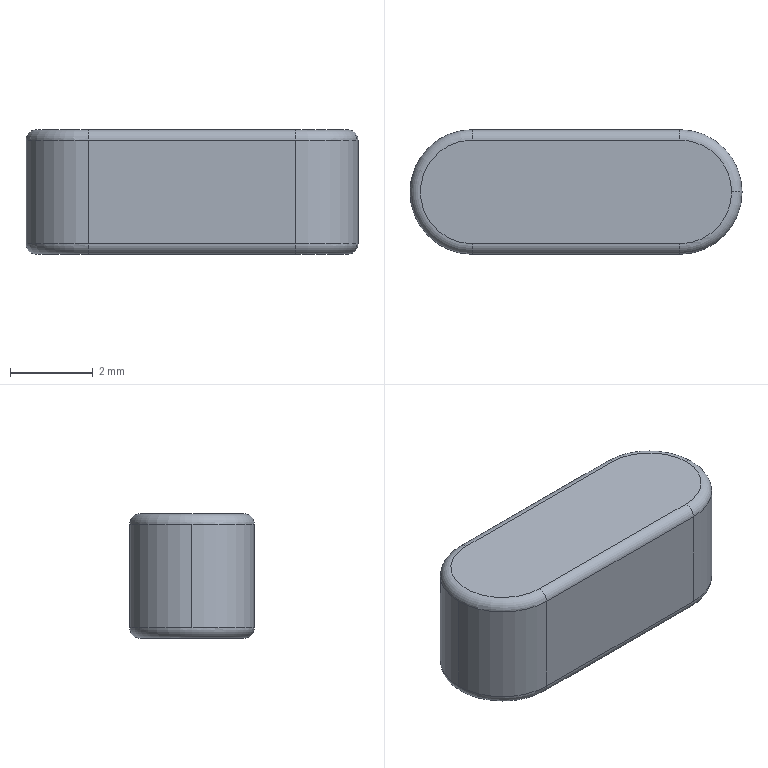Part | SolidWorks | features Extrusion 1, Fillet 1 | 1 solid | 17 faces | box 8 x 3 x 3 mm | volume 65.694 mm3 | cylinder 7 | torus 6 | plane 4 | commonest cylinder face diameters 0.5 x4 3 x3
STEP:
#1=CARTESIAN_POINT('',(3.75,0.,0.));
#2=VERTEX_POINT('',#1);
#3=CARTESIAN_POINT('',(2.5,-1.25,0.));
#4=VERTEX_POINT('',#3);
#5=CARTESIAN_POINT('',(2.5,0.,0.));
#6=DIRECTION('',(0.,0.,-1.));
#7=DIRECTION('',(1.,0.,0.));
#8=AXIS2_PLACEMENT_3D('',#5,#6,#7);
#9=CIRCLE('',#8,1.25);
#10=EDGE_CURVE('',#2,#4,#9,.T.);
#11=ORIENTED_EDGE('',*,*,#10,.F.);
#12=CARTESIAN_POINT('',(4.,0.,0.25));
#13=VERTEX_POINT('',#12);
#14=CARTESIAN_POINT('',(3.75,0.,0.25));
#15=DIRECTION('',(0.,-1.,0.));
#16=DIRECTION('',(0.,0.,-1.));
#17=AXIS2_PLACEMENT_3D('',#14,#15,#16);
#18=CIRCLE('',#17,0.25);
#19=EDGE_CURVE('',#2,#13,#18,.T.);
#20=ORIENTED_EDGE('',*,*,#19,.T.);
#21=CARTESIAN_POINT('',(2.5,-1.5,0.25));
#22=VERTEX_POINT('',#21);
#23=CARTESIAN_POINT('',(2.5,0.,0.25));
#24=DIRECTION('',(0.,0.,1.));
#25=DIRECTION('',(1.,0.,0.));
#26=AXIS2_PLACEMENT_3D('',#23,#24,#25);
#27=CIRCLE('',#26,1.5);
#28=EDGE_CURVE('',#22,#13,#27,.T.);
#29=ORIENTED_EDGE('',*,*,#28,.F.);
#30=CARTESIAN_POINT('',(2.5,-1.25,0.25));
#31=DIRECTION('',(1.,0.,0.));
#32=DIRECTION('',(0.,0.,-1.));
#33=AXIS2_PLACEMENT_3D('',#30,#31,#32);
#34=CIRCLE('',#33,0.25);
#35=EDGE_CURVE('',#22,#4,#34,.T.);
#36=ORIENTED_EDGE('',*,*,#35,.T.);
#37=EDGE_LOOP('',(#11,#20,#29,#36));
#38=FACE_OUTER_BOUND('',#37,.T.);
#39=CARTESIAN_POINT('',(2.5,0.,0.25));
#40=DIRECTION('',(0.,0.,1.));
#41=DIRECTION('',(1.,0.,0.));
#42=AXIS2_PLACEMENT_3D('',#39,#40,#41);
#43=TOROIDAL_SURFACE('',#42,1.25,0.25);
#44=ADVANCED_FACE('',(#38),#43,.T.);
#45=CARTESIAN_POINT('',(4.,0.,2.75));
#46=VERTEX_POINT('',#45);
#47=CARTESIAN_POINT('',(2.5,-1.5,2.75));
#48=VERTEX_POINT('',#47);
#49=CARTESIAN_POINT('',(2.5,0.,2.75));
#50=DIRECTION('',(0.,0.,-1.));
#51=DIRECTION('',(1.,0.,0.));
#52=AXIS2_PLACEMENT_3D('',#49,#50,#51);
#53=CIRCLE('',#52,1.5);
#54=EDGE_CURVE('',#46,#48,#53,.T.);
#55=ORIENTED_EDGE('',*,*,#54,.F.);
#56=CARTESIAN_POINT('',(3.75,0.,3.));
#57=VERTEX_POINT('',#56);
#58=CARTESIAN_POINT('',(3.75,0.,2.75));
#59=DIRECTION('',(0.,-1.,0.));
#60=DIRECTION('',(0.,0.,-1.));
#61=AXIS2_PLACEMENT_3D('',#58,#59,#60);
#62=CIRCLE('',#61,0.25);
#63=EDGE_CURVE('',#46,#57,#62,.T.);
#64=ORIENTED_EDGE('',*,*,#63,.T.);
#65=CARTESIAN_POINT('',(2.5,-1.25,3.));
#66=VERTEX_POINT('',#65);
#67=CARTESIAN_POINT('',(2.5,0.,3.));
#68=DIRECTION('',(0.,0.,1.));
#69=DIRECTION('',(1.,0.,0.));
#70=AXIS2_PLACEMENT_3D('',#67,#68,#69);
#71=CIRCLE('',#70,1.25);
#72=EDGE_CURVE('',#66,#57,#71,.T.);
#73=ORIENTED_EDGE('',*,*,#72,.F.);
#74=CARTESIAN_POINT('',(2.5,-1.25,2.75));
#75=DIRECTION('',(1.,0.,0.));
#76=DIRECTION('',(0.,0.,-1.));
#77=AXIS2_PLACEMENT_3D('',#74,#75,#76);
#78=CIRCLE('',#77,0.25);
#79=EDGE_CURVE('',#66,#48,#78,.T.);
#80=ORIENTED_EDGE('',*,*,#79,.T.);
#81=EDGE_LOOP('',(#55,#64,#73,#80));
#82=FACE_OUTER_BOUND('',#81,.T.);
#83=CARTESIAN_POINT('',(2.5,0.,2.75));
#84=DIRECTION('',(0.,0.,1.));
#85=DIRECTION('',(1.,0.,0.));
#86=AXIS2_PLACEMENT_3D('',#83,#84,#85);
#87=TOROIDAL_SURFACE('',#86,1.25,0.25);
#88=ADVANCED_FACE('',(#82),#87,.T.);
#89=CARTESIAN_POINT('',(-2.5,-1.5,2.75));
#90=VERTEX_POINT('',#89);
#91=CARTESIAN_POINT('',(-4.,0.,2.75));
#92=VERTEX_POINT('',#91);
#93=CARTESIAN_POINT('',(-2.5,0.,2.75));
#94=DIRECTION('',(0.,0.,-1.));
#95=DIRECTION('',(1.,0.,0.));
#96=AXIS2_PLACEMENT_3D('',#93,#94,#95);
#97=CIRCLE('',#96,1.5);
#98=EDGE_CURVE('',#90,#92,#97,.T.);
#99=ORIENTED_EDGE('',*,*,#98,.T.);
#100=CARTESIAN_POINT('',(-4.,0.,0.25));
#101=VERTEX_POINT('',#100);
#102=CARTESIAN_POINT('',(-4.,0.,3.));
#103=DIRECTION('',(0.,0.,-1.));
#104=VECTOR('',#103,1000.);
#105=LINE('',#102,#104);
#106=EDGE_CURVE('',#92,#101,#105,.T.);
#107=ORIENTED_EDGE('',*,*,#106,.T.);
#108=CARTESIAN_POINT('',(-2.5,-1.5,0.25));
#109=VERTEX_POINT('',#108);
#110=CARTESIAN_POINT('',(-2.5,0.,0.25));
#111=DIRECTION('',(0.,0.,1.));
#112=DIRECTION('',(1.,0.,0.));
#113=AXIS2_PLACEMENT_3D('',#110,#111,#112);
#114=CIRCLE('',#113,1.5);
#115=EDGE_CURVE('',#101,#109,#114,.T.);
#116=ORIENTED_EDGE('',*,*,#115,.T.);
#117=CARTESIAN_POINT('',(-2.5,-1.5,3.));
#118=DIRECTION('',(0.,0.,-1.));
#119=VECTOR('',#118,1000.);
#120=LINE('',#117,#119);
#121=EDGE_CURVE('',#90,#109,#120,.T.);
#122=ORIENTED_EDGE('',*,*,#121,.F.);
#123=EDGE_LOOP('',(#99,#107,#116,#122));
#124=FACE_OUTER_BOUND('',#123,.T.);
#125=CARTESIAN_POINT('',(-2.5,0.,3.));
#126=DIRECTION('',(0.,0.,-1.));
#127=DIRECTION('',(-1.,0.,0.));
#128=AXIS2_PLACEMENT_3D('',#125,#126,#127);
#129=CYLINDRICAL_SURFACE('',#128,1.5);
#130=ADVANCED_FACE('',(#124),#129,.T.);
#131=ORIENTED_EDGE('',*,*,#106,.F.);
#132=CARTESIAN_POINT('',(-2.5,1.5,2.75));
#133=VERTEX_POINT('',#132);
#134=CARTESIAN_POINT('',(-2.5,0.,2.75));
#135=DIRECTION('',(0.,0.,-1.));
#136=DIRECTION('',(1.,0.,0.));
#137=AXIS2_PLACEMENT_3D('',#134,#135,#136);
#138=CIRCLE('',#137,1.5);
#139=EDGE_CURVE('',#92,#133,#138,.T.);
#140=ORIENTED_EDGE('',*,*,#139,.T.);
#141=CARTESIAN_POINT('',(-2.5,1.5,0.25));
#142=VERTEX_POINT('',#141);
#143=CARTESIAN_POINT('',(-2.5,1.5,3.));
#144=DIRECTION('',(0.,0.,-1.));
#145=VECTOR('',#144,1000.);
#146=LINE('',#143,#145);
#147=EDGE_CURVE('',#133,#142,#146,.T.);
#148=ORIENTED_EDGE('',*,*,#147,.T.);
#149=CARTESIAN_POINT('',(-2.5,0.,0.25));
#150=DIRECTION('',(0.,0.,1.));
#151=DIRECTION('',(1.,0.,0.));
#152=AXIS2_PLACEMENT_3D('',#149,#150,#151);
#153=CIRCLE('',#152,1.5);
#154=EDGE_CURVE('',#142,#101,#153,.T.);
#155=ORIENTED_EDGE('',*,*,#154,.T.);
#156=EDGE_LOOP('',(#131,#140,#148,#155));
#157=FACE_OUTER_BOUND('',#156,.T.);
#158=CARTESIAN_POINT('',(-2.5,0.,3.));
#159=DIRECTION('',(0.,0.,-1.));
#160=DIRECTION('',(-1.,0.,0.));
#161=AXIS2_PLACEMENT_3D('',#158,#159,#160);
#162=CYLINDRICAL_SURFACE('',#161,1.5);
#163=ADVANCED_FACE('',(#157),#162,.T.);
#164=CARTESIAN_POINT('',(2.5,-1.5,3.));
#165=DIRECTION('',(0.,0.,-1.));
#166=VECTOR('',#165,1000.);
#167=LINE('',#164,#166);
#168=EDGE_CURVE('',#48,#22,#167,.T.);
#169=ORIENTED_EDGE('',*,*,#168,.F.);
#170=CARTESIAN_POINT('',(-2.5,-1.5,2.75));
#171=DIRECTION('',(-1.,0.,0.));
#172=VECTOR('',#171,1000.);
#173=LINE('',#170,#172);
#174=EDGE_CURVE('',#48,#90,#173,.T.);
#175=ORIENTED_EDGE('',*,*,#174,.T.);
#176=ORIENTED_EDGE('',*,*,#121,.T.);
#177=CARTESIAN_POINT('',(-2.5,-1.5,0.25));
#178=DIRECTION('',(1.,0.,0.));
#179=VECTOR('',#178,1000.);
#180=LINE('',#177,#179);
#181=EDGE_CURVE('',#109,#22,#180,.T.);
#182=ORIENTED_EDGE('',*,*,#181,.T.);
#183=EDGE_LOOP('',(#169,#175,#176,#182));
#184=FACE_OUTER_BOUND('',#183,.T.);
#185=CARTESIAN_POINT('',(-2.5,-1.5,3.));
#186=DIRECTION('',(0.,1.,0.));
#187=DIRECTION('',(-1.,0.,0.));
#188=AXIS2_PLACEMENT_3D('',#185,#186,#187);
#189=PLANE('',#188);
#190=ADVANCED_FACE('',(#184),#189,.F.);
#191=CARTESIAN_POINT('',(2.5,1.5,2.75));
#192=VERTEX_POINT('',#191);
#193=CARTESIAN_POINT('',(2.5,1.5,0.25));
#194=VERTEX_POINT('',#193);
#195=CARTESIAN_POINT('',(2.5,1.5,3.));
#196=DIRECTION('',(0.,0.,-1.));
#197=VECTOR('',#196,1000.);
#198=LINE('',#195,#197);
#199=EDGE_CURVE('',#192,#194,#198,.T.);
#200=ORIENTED_EDGE('',*,*,#199,.F.);
#201=CARTESIAN_POINT('',(2.5,0.,2.75));
#202=DIRECTION('',(0.,0.,-1.));
#203=DIRECTION('',(1.,0.,0.));
#204=AXIS2_PLACEMENT_3D('',#201,#202,#203);
#205=CIRCLE('',#204,1.5);
#206=EDGE_CURVE('',#192,#46,#205,.T.);
#207=ORIENTED_EDGE('',*,*,#206,.T.);
#208=ORIENTED_EDGE('',*,*,#54,.T.);
#209=ORIENTED_EDGE('',*,*,#168,.T.);
#210=ORIENTED_EDGE('',*,*,#28,.T.);
#211=CARTESIAN_POINT('',(2.5,0.,0.25));
#212=DIRECTION('',(0.,0.,1.));
#213=DIRECTION('',(1.,0.,0.));
#214=AXIS2_PLACEMENT_3D('',#211,#212,#213);
#215=CIRCLE('',#214,1.5);
#216=EDGE_CURVE('',#13,#194,#215,.T.);
#217=ORIENTED_EDGE('',*,*,#216,.T.);
#218=EDGE_LOOP('',(#200,#207,#208,#209,#210,#217));
#219=FACE_OUTER_BOUND('',#218,.T.);
#220=CARTESIAN_POINT('',(2.5,0.,3.));
#221=DIRECTION('',(0.,0.,-1.));
#222=DIRECTION('',(-1.,0.,0.));
#223=AXIS2_PLACEMENT_3D('',#220,#221,#222);
#224=CYLINDRICAL_SURFACE('',#223,1.5);
#225=ADVANCED_FACE('',(#219),#224,.T.);
#226=ORIENTED_EDGE('',*,*,#147,.F.);
#227=CARTESIAN_POINT('',(2.5,1.5,2.75));
#228=DIRECTION('',(1.,0.,0.));
#229=VECTOR('',#228,1000.);
#230=LINE('',#227,#229);
#231=EDGE_CURVE('',#133,#192,#230,.T.);
#232=ORIENTED_EDGE('',*,*,#231,.T.);
#233=ORIENTED_EDGE('',*,*,#199,.T.);
#234=CARTESIAN_POINT('',(-2.5,1.5,0.25));
#235=DIRECTION('',(-1.,0.,0.));
#236=VECTOR('',#235,1000.);
#237=LINE('',#234,#236);
#238=EDGE_CURVE('',#194,#142,#237,.T.);
#239=ORIENTED_EDGE('',*,*,#238,.T.);
#240=EDGE_LOOP('',(#226,#232,#233,#239));
#241=FACE_OUTER_BOUND('',#240,.T.);
#242=CARTESIAN_POINT('',(-2.5,1.5,3.));
#243=DIRECTION('',(0.,-1.,0.));
#244=DIRECTION('',(1.,0.,0.));
#245=AXIS2_PLACEMENT_3D('',#242,#243,#244);
#246=PLANE('',#245);
#247=ADVANCED_FACE('',(#241),#246,.F.);
#248=CARTESIAN_POINT('',(-2.5,-1.25,3.));
#249=VERTEX_POINT('',#248);
#250=CARTESIAN_POINT('',(2.5,-1.25,3.));
#251=DIRECTION('',(1.,0.,0.));
#252=VECTOR('',#251,1000.);
#253=LINE('',#250,#252);
#254=EDGE_CURVE('',#249,#66,#253,.T.);
#255=ORIENTED_EDGE('',*,*,#254,.T.);
#256=ORIENTED_EDGE('',*,*,#72,.T.);
#257=CARTESIAN_POINT('',(2.5,1.25,3.));
#258=VERTEX_POINT('',#257);
#259=CARTESIAN_POINT('',(2.5,0.,3.));
#260=DIRECTION('',(0.,0.,1.));
#261=DIRECTION('',(1.,0.,0.));
#262=AXIS2_PLACEMENT_3D('',#259,#260,#261);
#263=CIRCLE('',#262,1.25);
#264=EDGE_CURVE('',#57,#258,#263,.T.);
#265=ORIENTED_EDGE('',*,*,#264,.T.);
#266=CARTESIAN_POINT('',(-2.5,1.25,3.));
#267=VERTEX_POINT('',#266);
#268=CARTESIAN_POINT('',(-2.5,1.25,3.));
#269=DIRECTION('',(-1.,0.,0.));
#270=VECTOR('',#269,1000.);
#271=LINE('',#268,#270);
#272=EDGE_CURVE('',#258,#267,#271,.T.);
#273=ORIENTED_EDGE('',*,*,#272,.T.);
#274=CARTESIAN_POINT('',(-2.5,0.,3.));
#275=DIRECTION('',(0.,0.,1.));
#276=DIRECTION('',(1.,0.,0.));
#277=AXIS2_PLACEMENT_3D('',#274,#275,#276);
#278=CIRCLE('',#277,1.25);
#279=EDGE_CURVE('',#267,#249,#278,.T.);
#280=ORIENTED_EDGE('',*,*,#279,.T.);
#281=EDGE_LOOP('',(#255,#256,#265,#273,#280));
#282=FACE_OUTER_BOUND('',#281,.T.);
#283=CARTESIAN_POINT('',(-2.5,0.,3.));
#284=DIRECTION('',(0.,0.,1.));
#285=DIRECTION('',(1.,0.,0.));
#286=AXIS2_PLACEMENT_3D('',#283,#284,#285);
#287=PLANE('',#286);
#288=ADVANCED_FACE('',(#282),#287,.T.);
#289=CARTESIAN_POINT('',(-2.5,1.25,0.));
#290=VERTEX_POINT('',#289);
#291=CARTESIAN_POINT('',(2.5,1.25,0.));
#292=VERTEX_POINT('',#291);
#293=CARTESIAN_POINT('',(-2.5,1.25,0.));
#294=DIRECTION('',(1.,0.,0.));
#295=VECTOR('',#294,1000.);
#296=LINE('',#293,#295);
#297=EDGE_CURVE('',#290,#292,#296,.T.);
#298=ORIENTED_EDGE('',*,*,#297,.T.);
#299=CARTESIAN_POINT('',(2.5,0.,0.));
#300=DIRECTION('',(0.,0.,-1.));
#301=DIRECTION('',(1.,0.,0.));
#302=AXIS2_PLACEMENT_3D('',#299,#300,#301);
#303=CIRCLE('',#302,1.25);
#304=EDGE_CURVE('',#292,#2,#303,.T.);
#305=ORIENTED_EDGE('',*,*,#304,.T.);
#306=ORIENTED_EDGE('',*,*,#10,.T.);
#307=CARTESIAN_POINT('',(-2.5,-1.25,0.));
#308=VERTEX_POINT('',#307);
#309=CARTESIAN_POINT('',(-2.5,-1.25,0.));
#310=DIRECTION('',(-1.,0.,0.));
#311=VECTOR('',#310,1000.);
#312=LINE('',#309,#311);
#313=EDGE_CURVE('',#4,#308,#312,.T.);
#314=ORIENTED_EDGE('',*,*,#313,.T.);
#315=CARTESIAN_POINT('',(-2.5,0.,0.));
#316=DIRECTION('',(0.,0.,-1.));
#317=DIRECTION('',(1.,0.,0.));
#318=AXIS2_PLACEMENT_3D('',#315,#316,#317);
#319=CIRCLE('',#318,1.25);
#320=EDGE_CURVE('',#308,#290,#319,.T.);
#321=ORIENTED_EDGE('',*,*,#320,.T.);
#322=EDGE_LOOP('',(#298,#305,#306,#314,#321));
#323=FACE_OUTER_BOUND('',#322,.T.);
#324=CARTESIAN_POINT('',(-2.5,0.,0.));
#325=DIRECTION('',(0.,0.,1.));
#326=DIRECTION('',(1.,0.,0.));
#327=AXIS2_PLACEMENT_3D('',#324,#325,#326);
#328=PLANE('',#327);
#329=ADVANCED_FACE('',(#323),#328,.F.);
#330=CARTESIAN_POINT('',(-2.5,1.25,2.75));
#331=DIRECTION('',(1.,0.,0.));
#332=DIRECTION('',(0.,0.,-1.));
#333=AXIS2_PLACEMENT_3D('',#330,#331,#332);
#334=CIRCLE('',#333,0.25);
#335=EDGE_CURVE('',#133,#267,#334,.T.);
#336=ORIENTED_EDGE('',*,*,#335,.F.);
#337=ORIENTED_EDGE('',*,*,#139,.F.);
#338=ORIENTED_EDGE('',*,*,#98,.F.);
#339=CARTESIAN_POINT('',(-2.5,-1.25,2.75));
#340=DIRECTION('',(1.,0.,0.));
#341=DIRECTION('',(0.,0.,-1.));
#342=AXIS2_PLACEMENT_3D('',#339,#340,#341);
#343=CIRCLE('',#342,0.25);
#344=EDGE_CURVE('',#249,#90,#343,.T.);
#345=ORIENTED_EDGE('',*,*,#344,.F.);
#346=ORIENTED_EDGE('',*,*,#279,.F.);
#347=EDGE_LOOP('',(#336,#337,#338,#345,#346));
#348=FACE_OUTER_BOUND('',#347,.T.);
#349=CARTESIAN_POINT('',(-2.5,0.,2.75));
#350=DIRECTION('',(0.,0.,1.));
#351=DIRECTION('',(1.,0.,0.));
#352=AXIS2_PLACEMENT_3D('',#349,#350,#351);
#353=TOROIDAL_SURFACE('',#352,1.25,0.25);
#354=ADVANCED_FACE('',(#348),#353,.T.);
#355=ORIENTED_EDGE('',*,*,#344,.T.);
#356=ORIENTED_EDGE('',*,*,#174,.F.);
#357=ORIENTED_EDGE('',*,*,#79,.F.);
#358=ORIENTED_EDGE('',*,*,#254,.F.);
#359=EDGE_LOOP('',(#355,#356,#357,#358));
#360=FACE_OUTER_BOUND('',#359,.T.);
#361=CARTESIAN_POINT('',(-2.5,-1.25,2.75));
#362=DIRECTION('',(-1.,0.,0.));
#363=DIRECTION('',(0.,-1.,0.));
#364=AXIS2_PLACEMENT_3D('',#361,#362,#363);
#365=CYLINDRICAL_SURFACE('',#364,0.25);
#366=ADVANCED_FACE('',(#360),#365,.T.);
#367=ORIENTED_EDGE('',*,*,#335,.T.);
#368=ORIENTED_EDGE('',*,*,#272,.F.);
#369=CARTESIAN_POINT('',(2.5,1.25,2.75));
#370=DIRECTION('',(1.,0.,0.));
#371=DIRECTION('',(0.,0.,-1.));
#372=AXIS2_PLACEMENT_3D('',#369,#370,#371);
#373=CIRCLE('',#372,0.25);
#374=EDGE_CURVE('',#192,#258,#373,.T.);
#375=ORIENTED_EDGE('',*,*,#374,.F.);
#376=ORIENTED_EDGE('',*,*,#231,.F.);
#377=EDGE_LOOP('',(#367,#368,#375,#376));
#378=FACE_OUTER_BOUND('',#377,.T.);
#379=CARTESIAN_POINT('',(-2.5,1.25,2.75));
#380=DIRECTION('',(1.,0.,0.));
#381=DIRECTION('',(0.,1.,0.));
#382=AXIS2_PLACEMENT_3D('',#379,#380,#381);
#383=CYLINDRICAL_SURFACE('',#382,0.25);
#384=ADVANCED_FACE('',(#378),#383,.T.);
#385=ORIENTED_EDGE('',*,*,#63,.F.);
#386=ORIENTED_EDGE('',*,*,#206,.F.);
#387=ORIENTED_EDGE('',*,*,#374,.T.);
#388=ORIENTED_EDGE('',*,*,#264,.F.);
#389=EDGE_LOOP('',(#385,#386,#387,#388));
#390=FACE_OUTER_BOUND('',#389,.T.);
#391=CARTESIAN_POINT('',(2.5,0.,2.75));
#392=DIRECTION('',(0.,0.,1.));
#393=DIRECTION('',(1.,0.,0.));
#394=AXIS2_PLACEMENT_3D('',#391,#392,#393);
#395=TOROIDAL_SURFACE('',#394,1.25,0.25);
#396=ADVANCED_FACE('',(#390),#395,.T.);
#397=CARTESIAN_POINT('',(-2.5,1.25,0.25));
#398=DIRECTION('',(1.,0.,0.));
#399=DIRECTION('',(0.,0.,-1.));
#400=AXIS2_PLACEMENT_3D('',#397,#398,#399);
#401=CIRCLE('',#400,0.25);
#402=EDGE_CURVE('',#290,#142,#401,.T.);
#403=ORIENTED_EDGE('',*,*,#402,.F.);
#404=ORIENTED_EDGE('',*,*,#320,.F.);
#405=CARTESIAN_POINT('',(-2.5,-1.25,0.25));
#406=DIRECTION('',(1.,0.,0.));
#407=DIRECTION('',(0.,0.,-1.));
#408=AXIS2_PLACEMENT_3D('',#405,#406,#407);
#409=CIRCLE('',#408,0.25);
#410=EDGE_CURVE('',#109,#308,#409,.T.);
#411=ORIENTED_EDGE('',*,*,#410,.F.);
#412=ORIENTED_EDGE('',*,*,#115,.F.);
#413=ORIENTED_EDGE('',*,*,#154,.F.);
#414=EDGE_LOOP('',(#403,#404,#411,#412,#413));
#415=FACE_OUTER_BOUND('',#414,.T.);
#416=CARTESIAN_POINT('',(-2.5,0.,0.25));
#417=DIRECTION('',(0.,0.,1.));
#418=DIRECTION('',(1.,0.,0.));
#419=AXIS2_PLACEMENT_3D('',#416,#417,#418);
#420=TOROIDAL_SURFACE('',#419,1.25,0.25);
#421=ADVANCED_FACE('',(#415),#420,.T.);
#422=ORIENTED_EDGE('',*,*,#410,.T.);
#423=ORIENTED_EDGE('',*,*,#313,.F.);
#424=ORIENTED_EDGE('',*,*,#35,.F.);
#425=ORIENTED_EDGE('',*,*,#181,.F.);
#426=EDGE_LOOP('',(#422,#423,#424,#425));
#427=FACE_OUTER_BOUND('',#426,.T.);
#428=CARTESIAN_POINT('',(-2.5,-1.25,0.25));
#429=DIRECTION('',(1.,0.,0.));
#430=DIRECTION('',(0.,1.,0.));
#431=AXIS2_PLACEMENT_3D('',#428,#429,#430);
#432=CYLINDRICAL_SURFACE('',#431,0.25);
#433=ADVANCED_FACE('',(#427),#432,.T.);
#434=ORIENTED_EDGE('',*,*,#402,.T.);
#435=ORIENTED_EDGE('',*,*,#238,.F.);
#436=CARTESIAN_POINT('',(2.5,1.25,0.25));
#437=DIRECTION('',(1.,0.,0.));
#438=DIRECTION('',(0.,0.,-1.));
#439=AXIS2_PLACEMENT_3D('',#436,#437,#438);
#440=CIRCLE('',#439,0.25);
#441=EDGE_CURVE('',#292,#194,#440,.T.);
#442=ORIENTED_EDGE('',*,*,#441,.F.);
#443=ORIENTED_EDGE('',*,*,#297,.F.);
#444=EDGE_LOOP('',(#434,#435,#442,#443));
#445=FACE_OUTER_BOUND('',#444,.T.);
#446=CARTESIAN_POINT('',(-2.5,1.25,0.25));
#447=DIRECTION('',(-1.,0.,0.));
#448=DIRECTION('',(0.,-1.,0.));
#449=AXIS2_PLACEMENT_3D('',#446,#447,#448);
#450=CYLINDRICAL_SURFACE('',#449,0.25);
#451=ADVANCED_FACE('',(#445),#450,.T.);
#452=ORIENTED_EDGE('',*,*,#19,.F.);
#453=ORIENTED_EDGE('',*,*,#304,.F.);
#454=ORIENTED_EDGE('',*,*,#441,.T.);
#455=ORIENTED_EDGE('',*,*,#216,.F.);
#456=EDGE_LOOP('',(#452,#453,#454,#455));
#457=FACE_OUTER_BOUND('',#456,.T.);
#458=CARTESIAN_POINT('',(2.5,0.,0.25));
#459=DIRECTION('',(0.,0.,1.));
#460=DIRECTION('',(1.,0.,0.));
#461=AXIS2_PLACEMENT_3D('',#458,#459,#460);
#462=TOROIDAL_SURFACE('',#461,1.25,0.25);
#463=ADVANCED_FACE('',(#457),#462,.T.);
#464=CLOSED_SHELL('',(#44,#88,#130,#163,#190,#225,#247,#288,#329,#354,#366,#384,#396,#421,#433,#451,#463));
#465=MANIFOLD_SOLID_BREP('',#464);
#466=CARTESIAN_POINT('',(0.,0.,0.));
#467=DIRECTION('',(0.,0.,1.));
#468=DIRECTION('',(1.,0.,0.));
#469=AXIS2_PLACEMENT_3D('',#466,#467,#468);
#470=(LENGTH_UNIT()NAMED_UNIT(*)SI_UNIT(.MILLI.,.METRE.));
#471=UNCERTAINTY_MEASURE_WITH_UNIT(LENGTH_MEASURE(0.00001),#470,'','');
#472=(NAMED_UNIT(*)PLANE_ANGLE_UNIT()SI_UNIT($,.RADIAN.));
#473=(NAMED_UNIT(*)SI_UNIT($,.STERADIAN.)SOLID_ANGLE_UNIT());
#474=(GEOMETRIC_REPRESENTATION_CONTEXT(3)GLOBAL_UNCERTAINTY_ASSIGNED_CONTEXT((#471))GLOBAL_UNIT_ASSIGNED_CONTEXT((#470,#472,#473))REPRESENTATION_CONTEXT('',''));
#475=ADVANCED_BREP_SHAPE_REPRESENTATION('',(#465,#469),#474);